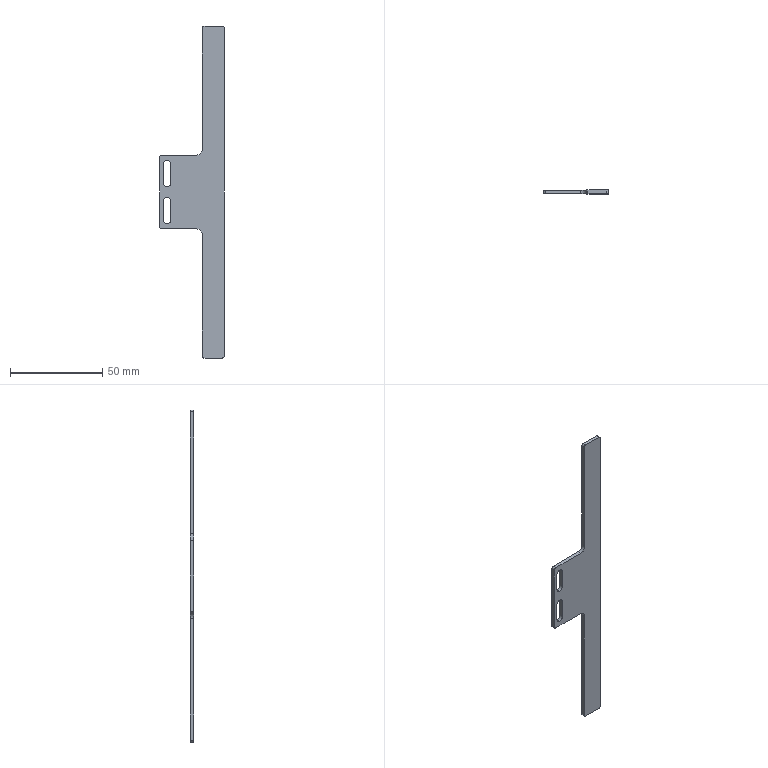Part | NX | features BREP 1 | 1 solid | 28 faces | box 35 x 2 x 180 mm | volume 5942 mm3 | plane 14 | cylinder 14 | commonest cylinder face diameters 2 x6 4.2 x6 6 x2
STEP:
#1=CARTESIAN_POINT('',(-28.9,0.,5.));
#2=VERTEX_POINT('',#1);
#3=CARTESIAN_POINT('',(-28.9,0.,15.));
#4=VERTEX_POINT('',#3);
#5=CARTESIAN_POINT('',(-28.9,0.,15.));
#6=DIRECTION('',(0.,0.,1.));
#7=VECTOR('',#6,1000.);
#8=LINE('',#5,#7);
#9=EDGE_CURVE('',#2,#4,#8,.T.);
#10=ORIENTED_EDGE('',*,*,#9,.T.);
#11=CARTESIAN_POINT('',(-28.9,2.,15.));
#12=VERTEX_POINT('',#11);
#13=CARTESIAN_POINT('',(-28.9,2.,15.));
#14=DIRECTION('',(0.,-1.,0.));
#15=VECTOR('',#14,1000.);
#16=LINE('',#13,#15);
#17=EDGE_CURVE('',#12,#4,#16,.T.);
#18=ORIENTED_EDGE('',*,*,#17,.F.);
#19=CARTESIAN_POINT('',(-28.9,2.,5.));
#20=VERTEX_POINT('',#19);
#21=CARTESIAN_POINT('',(-28.9,2.,15.));
#22=DIRECTION('',(0.,0.,1.));
#23=VECTOR('',#22,1000.);
#24=LINE('',#21,#23);
#25=EDGE_CURVE('',#20,#12,#24,.T.);
#26=ORIENTED_EDGE('',*,*,#25,.F.);
#27=CARTESIAN_POINT('',(-28.9,2.,5.));
#28=DIRECTION('',(0.,-1.,0.));
#29=VECTOR('',#28,1000.);
#30=LINE('',#27,#29);
#31=EDGE_CURVE('',#20,#2,#30,.T.);
#32=ORIENTED_EDGE('',*,*,#31,.T.);
#33=EDGE_LOOP('',(#10,#18,#26,#32));
#34=FACE_BOUND('',#33,.T.);
#35=CARTESIAN_POINT('',(-28.9,2.,15.));
#36=DIRECTION('',(1.,0.,0.));
#37=DIRECTION('',(0.,0.,-1.));
#38=AXIS2_PLACEMENT_3D('',#35,#36,#37);
#39=PLANE('',#38);
#40=ADVANCED_FACE('',(#34),#39,.F.);
#41=CARTESIAN_POINT('',(-33.1,0.,15.));
#42=VERTEX_POINT('',#41);
#43=CARTESIAN_POINT('',(-31.,0.,15.));
#44=DIRECTION('',(0.,-1.,0.));
#45=DIRECTION('',(0.,0.,1.));
#46=AXIS2_PLACEMENT_3D('',#43,#44,#45);
#47=CIRCLE('',#46,2.1);
#48=EDGE_CURVE('',#4,#42,#47,.T.);
#49=ORIENTED_EDGE('',*,*,#48,.T.);
#50=CARTESIAN_POINT('',(-33.1,2.,15.));
#51=VERTEX_POINT('',#50);
#52=CARTESIAN_POINT('',(-33.1,2.,15.));
#53=DIRECTION('',(0.,-1.,0.));
#54=VECTOR('',#53,1000.);
#55=LINE('',#52,#54);
#56=EDGE_CURVE('',#51,#42,#55,.T.);
#57=ORIENTED_EDGE('',*,*,#56,.F.);
#58=CARTESIAN_POINT('',(-31.,2.,15.));
#59=DIRECTION('',(0.,-1.,0.));
#60=DIRECTION('',(0.,0.,1.));
#61=AXIS2_PLACEMENT_3D('',#58,#59,#60);
#62=CIRCLE('',#61,2.1);
#63=EDGE_CURVE('',#12,#51,#62,.T.);
#64=ORIENTED_EDGE('',*,*,#63,.F.);
#65=ORIENTED_EDGE('',*,*,#17,.T.);
#66=EDGE_LOOP('',(#49,#57,#64,#65));
#67=FACE_BOUND('',#66,.T.);
#68=CARTESIAN_POINT('',(-31.,2.,15.));
#69=DIRECTION('',(0.,-1.,0.));
#70=DIRECTION('',(0.,0.,-1.));
#71=AXIS2_PLACEMENT_3D('',#68,#69,#70);
#72=CYLINDRICAL_SURFACE('',#71,2.1);
#73=ADVANCED_FACE('',(#67),#72,.F.);
#74=CARTESIAN_POINT('',(-33.1,0.,5.));
#75=VERTEX_POINT('',#74);
#76=CARTESIAN_POINT('',(-33.1,0.,5.));
#77=DIRECTION('',(0.,0.,-1.));
#78=VECTOR('',#77,1000.);
#79=LINE('',#76,#78);
#80=EDGE_CURVE('',#42,#75,#79,.T.);
#81=ORIENTED_EDGE('',*,*,#80,.T.);
#82=CARTESIAN_POINT('',(-33.1,2.,5.));
#83=VERTEX_POINT('',#82);
#84=CARTESIAN_POINT('',(-33.1,2.,5.));
#85=DIRECTION('',(0.,-1.,0.));
#86=VECTOR('',#85,1000.);
#87=LINE('',#84,#86);
#88=EDGE_CURVE('',#83,#75,#87,.T.);
#89=ORIENTED_EDGE('',*,*,#88,.F.);
#90=CARTESIAN_POINT('',(-33.1,2.,5.));
#91=DIRECTION('',(0.,0.,-1.));
#92=VECTOR('',#91,1000.);
#93=LINE('',#90,#92);
#94=EDGE_CURVE('',#51,#83,#93,.T.);
#95=ORIENTED_EDGE('',*,*,#94,.F.);
#96=ORIENTED_EDGE('',*,*,#56,.T.);
#97=EDGE_LOOP('',(#81,#89,#95,#96));
#98=FACE_BOUND('',#97,.T.);
#99=CARTESIAN_POINT('',(-33.1,2.,5.));
#100=DIRECTION('',(-1.,0.,0.));
#101=DIRECTION('',(0.,0.,1.));
#102=AXIS2_PLACEMENT_3D('',#99,#100,#101);
#103=PLANE('',#102);
#104=ADVANCED_FACE('',(#98),#103,.F.);
#105=CARTESIAN_POINT('',(-31.,2.,2.9));
#106=VERTEX_POINT('',#105);
#107=CARTESIAN_POINT('',(-31.,0.,2.9));
#108=VERTEX_POINT('',#107);
#109=CARTESIAN_POINT('',(-31.,2.,2.9));
#110=DIRECTION('',(0.,-1.,0.));
#111=VECTOR('',#110,1000.);
#112=LINE('',#109,#111);
#113=EDGE_CURVE('',#106,#108,#112,.T.);
#114=ORIENTED_EDGE('',*,*,#113,.F.);
#115=CARTESIAN_POINT('',(-31.,2.,5.));
#116=DIRECTION('',(0.,-1.,0.));
#117=DIRECTION('',(0.,0.,1.));
#118=AXIS2_PLACEMENT_3D('',#115,#116,#117);
#119=CIRCLE('',#118,2.1);
#120=EDGE_CURVE('',#83,#106,#119,.T.);
#121=ORIENTED_EDGE('',*,*,#120,.F.);
#122=ORIENTED_EDGE('',*,*,#88,.T.);
#123=CARTESIAN_POINT('',(-31.,0.,5.));
#124=DIRECTION('',(0.,-1.,0.));
#125=DIRECTION('',(0.,0.,1.));
#126=AXIS2_PLACEMENT_3D('',#123,#124,#125);
#127=CIRCLE('',#126,2.1);
#128=EDGE_CURVE('',#75,#108,#127,.T.);
#129=ORIENTED_EDGE('',*,*,#128,.T.);
#130=EDGE_LOOP('',(#114,#121,#122,#129));
#131=FACE_BOUND('',#130,.T.);
#132=CARTESIAN_POINT('',(-31.,2.,5.));
#133=DIRECTION('',(0.,-1.,0.));
#134=DIRECTION('',(0.,0.,-1.));
#135=AXIS2_PLACEMENT_3D('',#132,#133,#134);
#136=CYLINDRICAL_SURFACE('',#135,2.1);
#137=ADVANCED_FACE('',(#131),#136,.F.);
#138=CARTESIAN_POINT('',(-28.9,0.,-15.));
#139=VERTEX_POINT('',#138);
#140=CARTESIAN_POINT('',(-28.9,0.,-5.));
#141=VERTEX_POINT('',#140);
#142=CARTESIAN_POINT('',(-28.9,0.,-5.));
#143=DIRECTION('',(0.,0.,1.));
#144=VECTOR('',#143,1000.);
#145=LINE('',#142,#144);
#146=EDGE_CURVE('',#139,#141,#145,.T.);
#147=ORIENTED_EDGE('',*,*,#146,.T.);
#148=CARTESIAN_POINT('',(-28.9,2.,-5.));
#149=VERTEX_POINT('',#148);
#150=CARTESIAN_POINT('',(-28.9,2.,-5.));
#151=DIRECTION('',(0.,-1.,0.));
#152=VECTOR('',#151,1000.);
#153=LINE('',#150,#152);
#154=EDGE_CURVE('',#149,#141,#153,.T.);
#155=ORIENTED_EDGE('',*,*,#154,.F.);
#156=CARTESIAN_POINT('',(-28.9,2.,-15.));
#157=VERTEX_POINT('',#156);
#158=CARTESIAN_POINT('',(-28.9,2.,-5.));
#159=DIRECTION('',(0.,0.,1.));
#160=VECTOR('',#159,1000.);
#161=LINE('',#158,#160);
#162=EDGE_CURVE('',#157,#149,#161,.T.);
#163=ORIENTED_EDGE('',*,*,#162,.F.);
#164=CARTESIAN_POINT('',(-28.9,2.,-15.));
#165=DIRECTION('',(0.,-1.,0.));
#166=VECTOR('',#165,1000.);
#167=LINE('',#164,#166);
#168=EDGE_CURVE('',#157,#139,#167,.T.);
#169=ORIENTED_EDGE('',*,*,#168,.T.);
#170=EDGE_LOOP('',(#147,#155,#163,#169));
#171=FACE_BOUND('',#170,.T.);
#172=CARTESIAN_POINT('',(-28.9,2.,-5.));
#173=DIRECTION('',(1.,0.,0.));
#174=DIRECTION('',(0.,0.,-1.));
#175=AXIS2_PLACEMENT_3D('',#172,#173,#174);
#176=PLANE('',#175);
#177=ADVANCED_FACE('',(#171),#176,.F.);
#178=CARTESIAN_POINT('',(-33.1,0.,-5.));
#179=VERTEX_POINT('',#178);
#180=CARTESIAN_POINT('',(-31.,0.,-5.));
#181=DIRECTION('',(0.,-1.,0.));
#182=DIRECTION('',(0.,0.,1.));
#183=AXIS2_PLACEMENT_3D('',#180,#181,#182);
#184=CIRCLE('',#183,2.1);
#185=EDGE_CURVE('',#141,#179,#184,.T.);
#186=ORIENTED_EDGE('',*,*,#185,.T.);
#187=CARTESIAN_POINT('',(-33.1,2.,-5.));
#188=VERTEX_POINT('',#187);
#189=CARTESIAN_POINT('',(-33.1,2.,-5.));
#190=DIRECTION('',(0.,-1.,0.));
#191=VECTOR('',#190,1000.);
#192=LINE('',#189,#191);
#193=EDGE_CURVE('',#188,#179,#192,.T.);
#194=ORIENTED_EDGE('',*,*,#193,.F.);
#195=CARTESIAN_POINT('',(-31.,2.,-5.));
#196=DIRECTION('',(0.,-1.,0.));
#197=DIRECTION('',(0.,0.,1.));
#198=AXIS2_PLACEMENT_3D('',#195,#196,#197);
#199=CIRCLE('',#198,2.1);
#200=EDGE_CURVE('',#149,#188,#199,.T.);
#201=ORIENTED_EDGE('',*,*,#200,.F.);
#202=ORIENTED_EDGE('',*,*,#154,.T.);
#203=EDGE_LOOP('',(#186,#194,#201,#202));
#204=FACE_BOUND('',#203,.T.);
#205=CARTESIAN_POINT('',(-31.,2.,-5.));
#206=DIRECTION('',(0.,-1.,0.));
#207=DIRECTION('',(0.,0.,-1.));
#208=AXIS2_PLACEMENT_3D('',#205,#206,#207);
#209=CYLINDRICAL_SURFACE('',#208,2.1);
#210=ADVANCED_FACE('',(#204),#209,.F.);
#211=CARTESIAN_POINT('',(-33.1,0.,-15.));
#212=VERTEX_POINT('',#211);
#213=CARTESIAN_POINT('',(-33.1,0.,-15.));
#214=DIRECTION('',(0.,0.,-1.));
#215=VECTOR('',#214,1000.);
#216=LINE('',#213,#215);
#217=EDGE_CURVE('',#179,#212,#216,.T.);
#218=ORIENTED_EDGE('',*,*,#217,.T.);
#219=CARTESIAN_POINT('',(-33.1,2.,-15.));
#220=VERTEX_POINT('',#219);
#221=CARTESIAN_POINT('',(-33.1,2.,-15.));
#222=DIRECTION('',(0.,-1.,0.));
#223=VECTOR('',#222,1000.);
#224=LINE('',#221,#223);
#225=EDGE_CURVE('',#220,#212,#224,.T.);
#226=ORIENTED_EDGE('',*,*,#225,.F.);
#227=CARTESIAN_POINT('',(-33.1,2.,-15.));
#228=DIRECTION('',(0.,0.,-1.));
#229=VECTOR('',#228,1000.);
#230=LINE('',#227,#229);
#231=EDGE_CURVE('',#188,#220,#230,.T.);
#232=ORIENTED_EDGE('',*,*,#231,.F.);
#233=ORIENTED_EDGE('',*,*,#193,.T.);
#234=EDGE_LOOP('',(#218,#226,#232,#233));
#235=FACE_BOUND('',#234,.T.);
#236=CARTESIAN_POINT('',(-33.1,2.,-15.));
#237=DIRECTION('',(-1.,0.,0.));
#238=DIRECTION('',(0.,0.,1.));
#239=AXIS2_PLACEMENT_3D('',#236,#237,#238);
#240=PLANE('',#239);
#241=ADVANCED_FACE('',(#235),#240,.F.);
#242=CARTESIAN_POINT('',(-31.,2.,-17.1));
#243=VERTEX_POINT('',#242);
#244=CARTESIAN_POINT('',(-31.,0.,-17.1));
#245=VERTEX_POINT('',#244);
#246=CARTESIAN_POINT('',(-31.,2.,-17.1));
#247=DIRECTION('',(0.,-1.,0.));
#248=VECTOR('',#247,1000.);
#249=LINE('',#246,#248);
#250=EDGE_CURVE('',#243,#245,#249,.T.);
#251=ORIENTED_EDGE('',*,*,#250,.F.);
#252=CARTESIAN_POINT('',(-31.,2.,-15.));
#253=DIRECTION('',(0.,-1.,0.));
#254=DIRECTION('',(0.,0.,1.));
#255=AXIS2_PLACEMENT_3D('',#252,#253,#254);
#256=CIRCLE('',#255,2.1);
#257=EDGE_CURVE('',#220,#243,#256,.T.);
#258=ORIENTED_EDGE('',*,*,#257,.F.);
#259=ORIENTED_EDGE('',*,*,#225,.T.);
#260=CARTESIAN_POINT('',(-31.,0.,-15.));
#261=DIRECTION('',(0.,-1.,0.));
#262=DIRECTION('',(0.,0.,1.));
#263=AXIS2_PLACEMENT_3D('',#260,#261,#262);
#264=CIRCLE('',#263,2.1);
#265=EDGE_CURVE('',#212,#245,#264,.T.);
#266=ORIENTED_EDGE('',*,*,#265,.T.);
#267=EDGE_LOOP('',(#251,#258,#259,#266));
#268=FACE_BOUND('',#267,.T.);
#269=CARTESIAN_POINT('',(-31.,2.,-15.));
#270=DIRECTION('',(0.,-1.,0.));
#271=DIRECTION('',(0.,0.,-1.));
#272=AXIS2_PLACEMENT_3D('',#269,#270,#271);
#273=CYLINDRICAL_SURFACE('',#272,2.1);
#274=ADVANCED_FACE('',(#268),#273,.F.);
#275=CARTESIAN_POINT('',(-35.,0.,-19.));
#276=VERTEX_POINT('',#275);
#277=CARTESIAN_POINT('',(-34.,0.,-20.));
#278=VERTEX_POINT('',#277);
#279=CARTESIAN_POINT('',(-34.,0.,-19.));
#280=DIRECTION('',(0.,-1.,0.));
#281=DIRECTION('',(0.,0.,-1.));
#282=AXIS2_PLACEMENT_3D('',#279,#280,#281);
#283=CIRCLE('',#282,1.);
#284=EDGE_CURVE('',#276,#278,#283,.T.);
#285=ORIENTED_EDGE('',*,*,#284,.T.);
#286=CARTESIAN_POINT('',(-15.,0.,-20.));
#287=VERTEX_POINT('',#286);
#288=CARTESIAN_POINT('',(-34.,0.,-20.));
#289=DIRECTION('',(1.,0.,0.));
#290=VECTOR('',#289,1000.);
#291=LINE('',#288,#290);
#292=EDGE_CURVE('',#278,#287,#291,.T.);
#293=ORIENTED_EDGE('',*,*,#292,.T.);
#294=CARTESIAN_POINT('',(-12.,0.,-23.));
#295=VERTEX_POINT('',#294);
#296=CARTESIAN_POINT('',(-15.,0.,-23.));
#297=DIRECTION('',(0.,1.,0.));
#298=DIRECTION('',(0.,0.,1.));
#299=AXIS2_PLACEMENT_3D('',#296,#297,#298);
#300=CIRCLE('',#299,3.);
#301=EDGE_CURVE('',#287,#295,#300,.T.);
#302=ORIENTED_EDGE('',*,*,#301,.T.);
#303=CARTESIAN_POINT('',(-12.,0.,-89.));
#304=VERTEX_POINT('',#303);
#305=CARTESIAN_POINT('',(-12.,0.,-23.));
#306=DIRECTION('',(0.,0.,-1.));
#307=VECTOR('',#306,1000.);
#308=LINE('',#305,#307);
#309=EDGE_CURVE('',#295,#304,#308,.T.);
#310=ORIENTED_EDGE('',*,*,#309,.T.);
#311=CARTESIAN_POINT('',(-11.,0.,-90.));
#312=VERTEX_POINT('',#311);
#313=CARTESIAN_POINT('',(-11.,0.,-89.));
#314=DIRECTION('',(0.,-1.,0.));
#315=DIRECTION('',(0.,0.,-1.));
#316=AXIS2_PLACEMENT_3D('',#313,#314,#315);
#317=CIRCLE('',#316,1.);
#318=EDGE_CURVE('',#304,#312,#317,.T.);
#319=ORIENTED_EDGE('',*,*,#318,.T.);
#320=CARTESIAN_POINT('',(-1.,0.,-90.));
#321=VERTEX_POINT('',#320);
#322=CARTESIAN_POINT('',(-11.,0.,-90.));
#323=DIRECTION('',(1.,0.,0.));
#324=VECTOR('',#323,1000.);
#325=LINE('',#322,#324);
#326=EDGE_CURVE('',#312,#321,#325,.T.);
#327=ORIENTED_EDGE('',*,*,#326,.T.);
#328=CARTESIAN_POINT('',(0.,0.,-89.));
#329=VERTEX_POINT('',#328);
#330=CARTESIAN_POINT('',(-1.,0.,-89.));
#331=DIRECTION('',(0.,-1.,0.));
#332=DIRECTION('',(0.,0.,-1.));
#333=AXIS2_PLACEMENT_3D('',#330,#331,#332);
#334=CIRCLE('',#333,1.);
#335=EDGE_CURVE('',#321,#329,#334,.T.);
#336=ORIENTED_EDGE('',*,*,#335,.T.);
#337=CARTESIAN_POINT('',(0.,0.,89.));
#338=VERTEX_POINT('',#337);
#339=CARTESIAN_POINT('',(0.,0.,-89.));
#340=DIRECTION('',(0.,0.,1.));
#341=VECTOR('',#340,1000.);
#342=LINE('',#339,#341);
#343=EDGE_CURVE('',#329,#338,#342,.T.);
#344=ORIENTED_EDGE('',*,*,#343,.T.);
#345=CARTESIAN_POINT('',(-1.,0.,90.));
#346=VERTEX_POINT('',#345);
#347=CARTESIAN_POINT('',(-1.,0.,89.));
#348=DIRECTION('',(0.,-1.,0.));
#349=DIRECTION('',(0.,0.,-1.));
#350=AXIS2_PLACEMENT_3D('',#347,#348,#349);
#351=CIRCLE('',#350,1.);
#352=EDGE_CURVE('',#338,#346,#351,.T.);
#353=ORIENTED_EDGE('',*,*,#352,.T.);
#354=CARTESIAN_POINT('',(-11.,0.,90.));
#355=VERTEX_POINT('',#354);
#356=CARTESIAN_POINT('',(-1.,0.,90.));
#357=DIRECTION('',(-1.,0.,0.));
#358=VECTOR('',#357,1000.);
#359=LINE('',#356,#358);
#360=EDGE_CURVE('',#346,#355,#359,.T.);
#361=ORIENTED_EDGE('',*,*,#360,.T.);
#362=CARTESIAN_POINT('',(-12.,0.,89.));
#363=VERTEX_POINT('',#362);
#364=CARTESIAN_POINT('',(-11.,0.,89.));
#365=DIRECTION('',(0.,-1.,0.));
#366=DIRECTION('',(0.,0.,-1.));
#367=AXIS2_PLACEMENT_3D('',#364,#365,#366);
#368=CIRCLE('',#367,1.);
#369=EDGE_CURVE('',#355,#363,#368,.T.);
#370=ORIENTED_EDGE('',*,*,#369,.T.);
#371=CARTESIAN_POINT('',(-12.,0.,23.));
#372=VERTEX_POINT('',#371);
#373=CARTESIAN_POINT('',(-12.,0.,89.));
#374=DIRECTION('',(0.,0.,-1.));
#375=VECTOR('',#374,1000.);
#376=LINE('',#373,#375);
#377=EDGE_CURVE('',#363,#372,#376,.T.);
#378=ORIENTED_EDGE('',*,*,#377,.T.);
#379=CARTESIAN_POINT('',(-15.,0.,20.));
#380=VERTEX_POINT('',#379);
#381=CARTESIAN_POINT('',(-15.,0.,23.));
#382=DIRECTION('',(0.,1.,0.));
#383=DIRECTION('',(0.,0.,1.));
#384=AXIS2_PLACEMENT_3D('',#381,#382,#383);
#385=CIRCLE('',#384,3.);
#386=EDGE_CURVE('',#372,#380,#385,.T.);
#387=ORIENTED_EDGE('',*,*,#386,.T.);
#388=CARTESIAN_POINT('',(-34.,0.,20.));
#389=VERTEX_POINT('',#388);
#390=CARTESIAN_POINT('',(-15.,0.,20.));
#391=DIRECTION('',(-1.,0.,0.));
#392=VECTOR('',#391,1000.);
#393=LINE('',#390,#392);
#394=EDGE_CURVE('',#380,#389,#393,.T.);
#395=ORIENTED_EDGE('',*,*,#394,.T.);
#396=CARTESIAN_POINT('',(-35.,0.,19.));
#397=VERTEX_POINT('',#396);
#398=CARTESIAN_POINT('',(-34.,0.,19.));
#399=DIRECTION('',(0.,-1.,0.));
#400=DIRECTION('',(0.,0.,-1.));
#401=AXIS2_PLACEMENT_3D('',#398,#399,#400);
#402=CIRCLE('',#401,1.);
#403=EDGE_CURVE('',#389,#397,#402,.T.);
#404=ORIENTED_EDGE('',*,*,#403,.T.);
#405=CARTESIAN_POINT('',(-35.,0.,19.));
#406=DIRECTION('',(0.,0.,-1.));
#407=VECTOR('',#406,1000.);
#408=LINE('',#405,#407);
#409=EDGE_CURVE('',#397,#276,#408,.T.);
#410=ORIENTED_EDGE('',*,*,#409,.T.);
#411=EDGE_LOOP('',(#285,#293,#302,#310,#319,#327,#336,#344,#353,#361,#370,#378,#387,#395,#404,#410));
#412=FACE_BOUND('',#411,.T.);
#413=ORIENTED_EDGE('',*,*,#265,.F.);
#414=ORIENTED_EDGE('',*,*,#217,.F.);
#415=ORIENTED_EDGE('',*,*,#185,.F.);
#416=ORIENTED_EDGE('',*,*,#146,.F.);
#417=CARTESIAN_POINT('',(-31.,0.,-15.));
#418=DIRECTION('',(0.,-1.,0.));
#419=DIRECTION('',(0.,0.,1.));
#420=AXIS2_PLACEMENT_3D('',#417,#418,#419);
#421=CIRCLE('',#420,2.1);
#422=EDGE_CURVE('',#245,#139,#421,.T.);
#423=ORIENTED_EDGE('',*,*,#422,.F.);
#424=EDGE_LOOP('',(#413,#414,#415,#416,#423));
#425=FACE_BOUND('',#424,.T.);
#426=ORIENTED_EDGE('',*,*,#128,.F.);
#427=ORIENTED_EDGE('',*,*,#80,.F.);
#428=ORIENTED_EDGE('',*,*,#48,.F.);
#429=ORIENTED_EDGE('',*,*,#9,.F.);
#430=CARTESIAN_POINT('',(-31.,0.,5.));
#431=DIRECTION('',(0.,-1.,0.));
#432=DIRECTION('',(0.,0.,1.));
#433=AXIS2_PLACEMENT_3D('',#430,#431,#432);
#434=CIRCLE('',#433,2.1);
#435=EDGE_CURVE('',#108,#2,#434,.T.);
#436=ORIENTED_EDGE('',*,*,#435,.F.);
#437=EDGE_LOOP('',(#426,#427,#428,#429,#436));
#438=FACE_BOUND('',#437,.T.);
#439=CARTESIAN_POINT('',(-34.,0.,-19.));
#440=DIRECTION('',(0.,-1.,0.));
#441=DIRECTION('',(0.,0.,-1.));
#442=AXIS2_PLACEMENT_3D('',#439,#440,#441);
#443=PLANE('',#442);
#444=ADVANCED_FACE('',(#412,#425,#438),#443,.T.);
#445=CARTESIAN_POINT('',(-35.,2.,-19.));
#446=VERTEX_POINT('',#445);
#447=CARTESIAN_POINT('',(-34.,2.,-20.));
#448=VERTEX_POINT('',#447);
#449=CARTESIAN_POINT('',(-34.,2.,-19.));
#450=DIRECTION('',(0.,-1.,0.));
#451=DIRECTION('',(0.,0.,-1.));
#452=AXIS2_PLACEMENT_3D('',#449,#450,#451);
#453=CIRCLE('',#452,1.);
#454=EDGE_CURVE('',#446,#448,#453,.T.);
#455=ORIENTED_EDGE('',*,*,#454,.F.);
#456=CARTESIAN_POINT('',(-35.,2.,19.));
#457=VERTEX_POINT('',#456);
#458=CARTESIAN_POINT('',(-35.,2.,19.));
#459=DIRECTION('',(0.,0.,-1.));
#460=VECTOR('',#459,1000.);
#461=LINE('',#458,#460);
#462=EDGE_CURVE('',#457,#446,#461,.T.);
#463=ORIENTED_EDGE('',*,*,#462,.F.);
#464=CARTESIAN_POINT('',(-34.,2.,20.));
#465=VERTEX_POINT('',#464);
#466=CARTESIAN_POINT('',(-34.,2.,19.));
#467=DIRECTION('',(0.,-1.,0.));
#468=DIRECTION('',(0.,0.,-1.));
#469=AXIS2_PLACEMENT_3D('',#466,#467,#468);
#470=CIRCLE('',#469,1.);
#471=EDGE_CURVE('',#465,#457,#470,.T.);
#472=ORIENTED_EDGE('',*,*,#471,.F.);
#473=CARTESIAN_POINT('',(-15.,2.,20.));
#474=VERTEX_POINT('',#473);
#475=CARTESIAN_POINT('',(-15.,2.,20.));
#476=DIRECTION('',(-1.,0.,0.));
#477=VECTOR('',#476,1000.);
#478=LINE('',#475,#477);
#479=EDGE_CURVE('',#474,#465,#478,.T.);
#480=ORIENTED_EDGE('',*,*,#479,.F.);
#481=CARTESIAN_POINT('',(-12.,2.,23.));
#482=VERTEX_POINT('',#481);
#483=CARTESIAN_POINT('',(-15.,2.,23.));
#484=DIRECTION('',(0.,1.,0.));
#485=DIRECTION('',(0.,0.,1.));
#486=AXIS2_PLACEMENT_3D('',#483,#484,#485);
#487=CIRCLE('',#486,3.);
#488=EDGE_CURVE('',#482,#474,#487,.T.);
#489=ORIENTED_EDGE('',*,*,#488,.F.);
#490=CARTESIAN_POINT('',(-12.,2.,89.));
#491=VERTEX_POINT('',#490);
#492=CARTESIAN_POINT('',(-12.,2.,89.));
#493=DIRECTION('',(0.,0.,-1.));
#494=VECTOR('',#493,1000.);
#495=LINE('',#492,#494);
#496=EDGE_CURVE('',#491,#482,#495,.T.);
#497=ORIENTED_EDGE('',*,*,#496,.F.);
#498=CARTESIAN_POINT('',(-11.,2.,90.));
#499=VERTEX_POINT('',#498);
#500=CARTESIAN_POINT('',(-11.,2.,89.));
#501=DIRECTION('',(0.,-1.,0.));
#502=DIRECTION('',(0.,0.,-1.));
#503=AXIS2_PLACEMENT_3D('',#500,#501,#502);
#504=CIRCLE('',#503,1.);
#505=EDGE_CURVE('',#499,#491,#504,.T.);
#506=ORIENTED_EDGE('',*,*,#505,.F.);
#507=CARTESIAN_POINT('',(-1.,2.,90.));
#508=VERTEX_POINT('',#507);
#509=CARTESIAN_POINT('',(-1.,2.,90.));
#510=DIRECTION('',(-1.,0.,0.));
#511=VECTOR('',#510,1000.);
#512=LINE('',#509,#511);
#513=EDGE_CURVE('',#508,#499,#512,.T.);
#514=ORIENTED_EDGE('',*,*,#513,.F.);
#515=CARTESIAN_POINT('',(0.,2.,89.));
#516=VERTEX_POINT('',#515);
#517=CARTESIAN_POINT('',(-1.,2.,89.));
#518=DIRECTION('',(0.,-1.,0.));
#519=DIRECTION('',(0.,0.,-1.));
#520=AXIS2_PLACEMENT_3D('',#517,#518,#519);
#521=CIRCLE('',#520,1.);
#522=EDGE_CURVE('',#516,#508,#521,.T.);
#523=ORIENTED_EDGE('',*,*,#522,.F.);
#524=CARTESIAN_POINT('',(0.,2.,-89.));
#525=VERTEX_POINT('',#524);
#526=CARTESIAN_POINT('',(0.,2.,-89.));
#527=DIRECTION('',(0.,0.,1.));
#528=VECTOR('',#527,1000.);
#529=LINE('',#526,#528);
#530=EDGE_CURVE('',#525,#516,#529,.T.);
#531=ORIENTED_EDGE('',*,*,#530,.F.);
#532=CARTESIAN_POINT('',(-1.,2.,-90.));
#533=VERTEX_POINT('',#532);
#534=CARTESIAN_POINT('',(-1.,2.,-89.));
#535=DIRECTION('',(0.,-1.,0.));
#536=DIRECTION('',(0.,0.,-1.));
#537=AXIS2_PLACEMENT_3D('',#534,#535,#536);
#538=CIRCLE('',#537,1.);
#539=EDGE_CURVE('',#533,#525,#538,.T.);
#540=ORIENTED_EDGE('',*,*,#539,.F.);
#541=CARTESIAN_POINT('',(-11.,2.,-90.));
#542=VERTEX_POINT('',#541);
#543=CARTESIAN_POINT('',(-11.,2.,-90.));
#544=DIRECTION('',(1.,0.,0.));
#545=VECTOR('',#544,1000.);
#546=LINE('',#543,#545);
#547=EDGE_CURVE('',#542,#533,#546,.T.);
#548=ORIENTED_EDGE('',*,*,#547,.F.);
#549=CARTESIAN_POINT('',(-12.,2.,-89.));
#550=VERTEX_POINT('',#549);
#551=CARTESIAN_POINT('',(-11.,2.,-89.));
#552=DIRECTION('',(0.,-1.,0.));
#553=DIRECTION('',(0.,0.,-1.));
#554=AXIS2_PLACEMENT_3D('',#551,#552,#553);
#555=CIRCLE('',#554,1.);
#556=EDGE_CURVE('',#550,#542,#555,.T.);
#557=ORIENTED_EDGE('',*,*,#556,.F.);
#558=CARTESIAN_POINT('',(-12.,2.,-23.));
#559=VERTEX_POINT('',#558);
#560=CARTESIAN_POINT('',(-12.,2.,-23.));
#561=DIRECTION('',(0.,0.,-1.));
#562=VECTOR('',#561,1000.);
#563=LINE('',#560,#562);
#564=EDGE_CURVE('',#559,#550,#563,.T.);
#565=ORIENTED_EDGE('',*,*,#564,.F.);
#566=CARTESIAN_POINT('',(-15.,2.,-20.));
#567=VERTEX_POINT('',#566);
#568=CARTESIAN_POINT('',(-15.,2.,-23.));
#569=DIRECTION('',(0.,1.,0.));
#570=DIRECTION('',(0.,0.,1.));
#571=AXIS2_PLACEMENT_3D('',#568,#569,#570);
#572=CIRCLE('',#571,3.);
#573=EDGE_CURVE('',#567,#559,#572,.T.);
#574=ORIENTED_EDGE('',*,*,#573,.F.);
#575=CARTESIAN_POINT('',(-34.,2.,-20.));
#576=DIRECTION('',(1.,0.,0.));
#577=VECTOR('',#576,1000.);
#578=LINE('',#575,#577);
#579=EDGE_CURVE('',#448,#567,#578,.T.);
#580=ORIENTED_EDGE('',*,*,#579,.F.);
#581=EDGE_LOOP('',(#455,#463,#472,#480,#489,#497,#506,#514,#523,#531,#540,#548,#557,#565,#574,#580));
#582=FACE_BOUND('',#581,.T.);
#583=ORIENTED_EDGE('',*,*,#231,.T.);
#584=ORIENTED_EDGE('',*,*,#257,.T.);
#585=CARTESIAN_POINT('',(-31.,2.,-15.));
#586=DIRECTION('',(0.,-1.,0.));
#587=DIRECTION('',(0.,0.,1.));
#588=AXIS2_PLACEMENT_3D('',#585,#586,#587);
#589=CIRCLE('',#588,2.1);
#590=EDGE_CURVE('',#243,#157,#589,.T.);
#591=ORIENTED_EDGE('',*,*,#590,.T.);
#592=ORIENTED_EDGE('',*,*,#162,.T.);
#593=ORIENTED_EDGE('',*,*,#200,.T.);
#594=EDGE_LOOP('',(#583,#584,#591,#592,#593));
#595=FACE_BOUND('',#594,.T.);
#596=ORIENTED_EDGE('',*,*,#94,.T.);
#597=ORIENTED_EDGE('',*,*,#120,.T.);
#598=CARTESIAN_POINT('',(-31.,2.,5.));
#599=DIRECTION('',(0.,-1.,0.));
#600=DIRECTION('',(0.,0.,1.));
#601=AXIS2_PLACEMENT_3D('',#598,#599,#600);
#602=CIRCLE('',#601,2.1);
#603=EDGE_CURVE('',#106,#20,#602,.T.);
#604=ORIENTED_EDGE('',*,*,#603,.T.);
#605=ORIENTED_EDGE('',*,*,#25,.T.);
#606=ORIENTED_EDGE('',*,*,#63,.T.);
#607=EDGE_LOOP('',(#596,#597,#604,#605,#606));
#608=FACE_BOUND('',#607,.T.);
#609=CARTESIAN_POINT('',(-34.,2.,-19.));
#610=DIRECTION('',(0.,-1.,0.));
#611=DIRECTION('',(0.,0.,-1.));
#612=AXIS2_PLACEMENT_3D('',#609,#610,#611);
#613=PLANE('',#612);
#614=ADVANCED_FACE('',(#582,#595,#608),#613,.F.);
#615=ORIENTED_EDGE('',*,*,#292,.F.);
#616=CARTESIAN_POINT('',(-34.,2.,-20.));
#617=DIRECTION('',(0.,-1.,0.));
#618=VECTOR('',#617,1000.);
#619=LINE('',#616,#618);
#620=EDGE_CURVE('',#448,#278,#619,.T.);
#621=ORIENTED_EDGE('',*,*,#620,.F.);
#622=ORIENTED_EDGE('',*,*,#579,.T.);
#623=CARTESIAN_POINT('',(-15.,2.,-20.));
#624=DIRECTION('',(0.,-1.,0.));
#625=VECTOR('',#624,1000.);
#626=LINE('',#623,#625);
#627=EDGE_CURVE('',#567,#287,#626,.T.);
#628=ORIENTED_EDGE('',*,*,#627,.T.);
#629=EDGE_LOOP('',(#615,#621,#622,#628));
#630=FACE_BOUND('',#629,.T.);
#631=CARTESIAN_POINT('',(-34.,2.,-20.));
#632=DIRECTION('',(0.,0.,-1.));
#633=DIRECTION('',(-1.,0.,0.));
#634=AXIS2_PLACEMENT_3D('',#631,#632,#633);
#635=PLANE('',#634);
#636=ADVANCED_FACE('',(#630),#635,.T.);
#637=ORIENTED_EDGE('',*,*,#301,.F.);
#638=ORIENTED_EDGE('',*,*,#627,.F.);
#639=ORIENTED_EDGE('',*,*,#573,.T.);
#640=CARTESIAN_POINT('',(-12.,2.,-23.));
#641=DIRECTION('',(0.,-1.,0.));
#642=VECTOR('',#641,1000.);
#643=LINE('',#640,#642);
#644=EDGE_CURVE('',#559,#295,#643,.T.);
#645=ORIENTED_EDGE('',*,*,#644,.T.);
#646=EDGE_LOOP('',(#637,#638,#639,#645));
#647=FACE_BOUND('',#646,.T.);
#648=CARTESIAN_POINT('',(-15.,2.,-23.));
#649=DIRECTION('',(0.,-1.,0.));
#650=DIRECTION('',(0.,0.,-1.));
#651=AXIS2_PLACEMENT_3D('',#648,#649,#650);
#652=CYLINDRICAL_SURFACE('',#651,3.);
#653=ADVANCED_FACE('',(#647),#652,.F.);
#654=ORIENTED_EDGE('',*,*,#309,.F.);
#655=ORIENTED_EDGE('',*,*,#644,.F.);
#656=ORIENTED_EDGE('',*,*,#564,.T.);
#657=CARTESIAN_POINT('',(-12.,2.,-89.));
#658=DIRECTION('',(0.,-1.,0.));
#659=VECTOR('',#658,1000.);
#660=LINE('',#657,#659);
#661=EDGE_CURVE('',#550,#304,#660,.T.);
#662=ORIENTED_EDGE('',*,*,#661,.T.);
#663=EDGE_LOOP('',(#654,#655,#656,#662));
#664=FACE_BOUND('',#663,.T.);
#665=CARTESIAN_POINT('',(-12.,2.,-23.));
#666=DIRECTION('',(-1.,0.,0.));
#667=DIRECTION('',(0.,0.,1.));
#668=AXIS2_PLACEMENT_3D('',#665,#666,#667);
#669=PLANE('',#668);
#670=ADVANCED_FACE('',(#664),#669,.T.);
#671=ORIENTED_EDGE('',*,*,#318,.F.);
#672=ORIENTED_EDGE('',*,*,#661,.F.);
#673=ORIENTED_EDGE('',*,*,#556,.T.);
#674=CARTESIAN_POINT('',(-11.,2.,-90.));
#675=DIRECTION('',(0.,-1.,0.));
#676=VECTOR('',#675,1000.);
#677=LINE('',#674,#676);
#678=EDGE_CURVE('',#542,#312,#677,.T.);
#679=ORIENTED_EDGE('',*,*,#678,.T.);
#680=EDGE_LOOP('',(#671,#672,#673,#679));
#681=FACE_BOUND('',#680,.T.);
#682=CARTESIAN_POINT('',(-11.,2.,-89.));
#683=DIRECTION('',(0.,-1.,0.));
#684=DIRECTION('',(0.,0.,-1.));
#685=AXIS2_PLACEMENT_3D('',#682,#683,#684);
#686=CYLINDRICAL_SURFACE('',#685,1.);
#687=ADVANCED_FACE('',(#681),#686,.T.);
#688=ORIENTED_EDGE('',*,*,#326,.F.);
#689=ORIENTED_EDGE('',*,*,#678,.F.);
#690=ORIENTED_EDGE('',*,*,#547,.T.);
#691=CARTESIAN_POINT('',(-1.,2.,-90.));
#692=DIRECTION('',(0.,-1.,0.));
#693=VECTOR('',#692,1000.);
#694=LINE('',#691,#693);
#695=EDGE_CURVE('',#533,#321,#694,.T.);
#696=ORIENTED_EDGE('',*,*,#695,.T.);
#697=EDGE_LOOP('',(#688,#689,#690,#696));
#698=FACE_BOUND('',#697,.T.);
#699=CARTESIAN_POINT('',(-11.,2.,-90.));
#700=DIRECTION('',(0.,0.,-1.));
#701=DIRECTION('',(-1.,0.,0.));
#702=AXIS2_PLACEMENT_3D('',#699,#700,#701);
#703=PLANE('',#702);
#704=ADVANCED_FACE('',(#698),#703,.T.);
#705=ORIENTED_EDGE('',*,*,#335,.F.);
#706=ORIENTED_EDGE('',*,*,#695,.F.);
#707=ORIENTED_EDGE('',*,*,#539,.T.);
#708=CARTESIAN_POINT('',(0.,2.,-89.));
#709=DIRECTION('',(0.,-1.,0.));
#710=VECTOR('',#709,1000.);
#711=LINE('',#708,#710);
#712=EDGE_CURVE('',#525,#329,#711,.T.);
#713=ORIENTED_EDGE('',*,*,#712,.T.);
#714=EDGE_LOOP('',(#705,#706,#707,#713));
#715=FACE_BOUND('',#714,.T.);
#716=CARTESIAN_POINT('',(-1.,2.,-89.));
#717=DIRECTION('',(0.,-1.,0.));
#718=DIRECTION('',(0.,0.,-1.));
#719=AXIS2_PLACEMENT_3D('',#716,#717,#718);
#720=CYLINDRICAL_SURFACE('',#719,1.);
#721=ADVANCED_FACE('',(#715),#720,.T.);
#722=ORIENTED_EDGE('',*,*,#343,.F.);
#723=ORIENTED_EDGE('',*,*,#712,.F.);
#724=ORIENTED_EDGE('',*,*,#530,.T.);
#725=CARTESIAN_POINT('',(0.,2.,89.));
#726=DIRECTION('',(0.,-1.,0.));
#727=VECTOR('',#726,1000.);
#728=LINE('',#725,#727);
#729=EDGE_CURVE('',#516,#338,#728,.T.);
#730=ORIENTED_EDGE('',*,*,#729,.T.);
#731=EDGE_LOOP('',(#722,#723,#724,#730));
#732=FACE_BOUND('',#731,.T.);
#733=CARTESIAN_POINT('',(0.,2.,-89.));
#734=DIRECTION('',(1.,0.,0.));
#735=DIRECTION('',(0.,0.,-1.));
#736=AXIS2_PLACEMENT_3D('',#733,#734,#735);
#737=PLANE('',#736);
#738=ADVANCED_FACE('',(#732),#737,.T.);
#739=ORIENTED_EDGE('',*,*,#352,.F.);
#740=ORIENTED_EDGE('',*,*,#729,.F.);
#741=ORIENTED_EDGE('',*,*,#522,.T.);
#742=CARTESIAN_POINT('',(-1.,2.,90.));
#743=DIRECTION('',(0.,-1.,0.));
#744=VECTOR('',#743,1000.);
#745=LINE('',#742,#744);
#746=EDGE_CURVE('',#508,#346,#745,.T.);
#747=ORIENTED_EDGE('',*,*,#746,.T.);
#748=EDGE_LOOP('',(#739,#740,#741,#747));
#749=FACE_BOUND('',#748,.T.);
#750=CARTESIAN_POINT('',(-1.,2.,89.));
#751=DIRECTION('',(0.,-1.,0.));
#752=DIRECTION('',(0.,0.,-1.));
#753=AXIS2_PLACEMENT_3D('',#750,#751,#752);
#754=CYLINDRICAL_SURFACE('',#753,1.);
#755=ADVANCED_FACE('',(#749),#754,.T.);
#756=ORIENTED_EDGE('',*,*,#360,.F.);
#757=ORIENTED_EDGE('',*,*,#746,.F.);
#758=ORIENTED_EDGE('',*,*,#513,.T.);
#759=CARTESIAN_POINT('',(-11.,2.,90.));
#760=DIRECTION('',(0.,-1.,0.));
#761=VECTOR('',#760,1000.);
#762=LINE('',#759,#761);
#763=EDGE_CURVE('',#499,#355,#762,.T.);
#764=ORIENTED_EDGE('',*,*,#763,.T.);
#765=EDGE_LOOP('',(#756,#757,#758,#764));
#766=FACE_BOUND('',#765,.T.);
#767=CARTESIAN_POINT('',(-1.,2.,90.));
#768=DIRECTION('',(0.,0.,1.));
#769=DIRECTION('',(1.,0.,0.));
#770=AXIS2_PLACEMENT_3D('',#767,#768,#769);
#771=PLANE('',#770);
#772=ADVANCED_FACE('',(#766),#771,.T.);
#773=ORIENTED_EDGE('',*,*,#369,.F.);
#774=ORIENTED_EDGE('',*,*,#763,.F.);
#775=ORIENTED_EDGE('',*,*,#505,.T.);
#776=CARTESIAN_POINT('',(-12.,2.,89.));
#777=DIRECTION('',(0.,-1.,0.));
#778=VECTOR('',#777,1000.);
#779=LINE('',#776,#778);
#780=EDGE_CURVE('',#491,#363,#779,.T.);
#781=ORIENTED_EDGE('',*,*,#780,.T.);
#782=EDGE_LOOP('',(#773,#774,#775,#781));
#783=FACE_BOUND('',#782,.T.);
#784=CARTESIAN_POINT('',(-11.,2.,89.));
#785=DIRECTION('',(0.,-1.,0.));
#786=DIRECTION('',(0.,0.,-1.));
#787=AXIS2_PLACEMENT_3D('',#784,#785,#786);
#788=CYLINDRICAL_SURFACE('',#787,1.);
#789=ADVANCED_FACE('',(#783),#788,.T.);
#790=ORIENTED_EDGE('',*,*,#377,.F.);
#791=ORIENTED_EDGE('',*,*,#780,.F.);
#792=ORIENTED_EDGE('',*,*,#496,.T.);
#793=CARTESIAN_POINT('',(-12.,2.,23.));
#794=DIRECTION('',(0.,-1.,0.));
#795=VECTOR('',#794,1000.);
#796=LINE('',#793,#795);
#797=EDGE_CURVE('',#482,#372,#796,.T.);
#798=ORIENTED_EDGE('',*,*,#797,.T.);
#799=EDGE_LOOP('',(#790,#791,#792,#798));
#800=FACE_BOUND('',#799,.T.);
#801=CARTESIAN_POINT('',(-12.,2.,89.));
#802=DIRECTION('',(-1.,0.,0.));
#803=DIRECTION('',(0.,0.,1.));
#804=AXIS2_PLACEMENT_3D('',#801,#802,#803);
#805=PLANE('',#804);
#806=ADVANCED_FACE('',(#800),#805,.T.);
#807=ORIENTED_EDGE('',*,*,#386,.F.);
#808=ORIENTED_EDGE('',*,*,#797,.F.);
#809=ORIENTED_EDGE('',*,*,#488,.T.);
#810=CARTESIAN_POINT('',(-15.,2.,20.));
#811=DIRECTION('',(0.,-1.,0.));
#812=VECTOR('',#811,1000.);
#813=LINE('',#810,#812);
#814=EDGE_CURVE('',#474,#380,#813,.T.);
#815=ORIENTED_EDGE('',*,*,#814,.T.);
#816=EDGE_LOOP('',(#807,#808,#809,#815));
#817=FACE_BOUND('',#816,.T.);
#818=CARTESIAN_POINT('',(-15.,2.,23.));
#819=DIRECTION('',(0.,-1.,0.));
#820=DIRECTION('',(0.,0.,-1.));
#821=AXIS2_PLACEMENT_3D('',#818,#819,#820);
#822=CYLINDRICAL_SURFACE('',#821,3.);
#823=ADVANCED_FACE('',(#817),#822,.F.);
#824=ORIENTED_EDGE('',*,*,#394,.F.);
#825=ORIENTED_EDGE('',*,*,#814,.F.);
#826=ORIENTED_EDGE('',*,*,#479,.T.);
#827=CARTESIAN_POINT('',(-34.,2.,20.));
#828=DIRECTION('',(0.,-1.,0.));
#829=VECTOR('',#828,1000.);
#830=LINE('',#827,#829);
#831=EDGE_CURVE('',#465,#389,#830,.T.);
#832=ORIENTED_EDGE('',*,*,#831,.T.);
#833=EDGE_LOOP('',(#824,#825,#826,#832));
#834=FACE_BOUND('',#833,.T.);
#835=CARTESIAN_POINT('',(-15.,2.,20.));
#836=DIRECTION('',(0.,0.,1.));
#837=DIRECTION('',(1.,0.,0.));
#838=AXIS2_PLACEMENT_3D('',#835,#836,#837);
#839=PLANE('',#838);
#840=ADVANCED_FACE('',(#834),#839,.T.);
#841=ORIENTED_EDGE('',*,*,#403,.F.);
#842=ORIENTED_EDGE('',*,*,#831,.F.);
#843=ORIENTED_EDGE('',*,*,#471,.T.);
#844=CARTESIAN_POINT('',(-35.,2.,19.));
#845=DIRECTION('',(0.,-1.,0.));
#846=VECTOR('',#845,1000.);
#847=LINE('',#844,#846);
#848=EDGE_CURVE('',#457,#397,#847,.T.);
#849=ORIENTED_EDGE('',*,*,#848,.T.);
#850=EDGE_LOOP('',(#841,#842,#843,#849));
#851=FACE_BOUND('',#850,.T.);
#852=CARTESIAN_POINT('',(-34.,2.,19.));
#853=DIRECTION('',(0.,-1.,0.));
#854=DIRECTION('',(0.,0.,-1.));
#855=AXIS2_PLACEMENT_3D('',#852,#853,#854);
#856=CYLINDRICAL_SURFACE('',#855,1.);
#857=ADVANCED_FACE('',(#851),#856,.T.);
#858=ORIENTED_EDGE('',*,*,#409,.F.);
#859=ORIENTED_EDGE('',*,*,#848,.F.);
#860=ORIENTED_EDGE('',*,*,#462,.T.);
#861=CARTESIAN_POINT('',(-35.,2.,-19.));
#862=DIRECTION('',(0.,-1.,0.));
#863=VECTOR('',#862,1000.);
#864=LINE('',#861,#863);
#865=EDGE_CURVE('',#446,#276,#864,.T.);
#866=ORIENTED_EDGE('',*,*,#865,.T.);
#867=EDGE_LOOP('',(#858,#859,#860,#866));
#868=FACE_BOUND('',#867,.T.);
#869=CARTESIAN_POINT('',(-35.,2.,19.));
#870=DIRECTION('',(-1.,0.,0.));
#871=DIRECTION('',(0.,0.,1.));
#872=AXIS2_PLACEMENT_3D('',#869,#870,#871);
#873=PLANE('',#872);
#874=ADVANCED_FACE('',(#868),#873,.T.);
#875=ORIENTED_EDGE('',*,*,#284,.F.);
#876=ORIENTED_EDGE('',*,*,#865,.F.);
#877=ORIENTED_EDGE('',*,*,#454,.T.);
#878=ORIENTED_EDGE('',*,*,#620,.T.);
#879=EDGE_LOOP('',(#875,#876,#877,#878));
#880=FACE_BOUND('',#879,.T.);
#881=CARTESIAN_POINT('',(-34.,2.,-19.));
#882=DIRECTION('',(0.,-1.,0.));
#883=DIRECTION('',(0.,0.,-1.));
#884=AXIS2_PLACEMENT_3D('',#881,#882,#883);
#885=CYLINDRICAL_SURFACE('',#884,1.);
#886=ADVANCED_FACE('',(#880),#885,.T.);
#887=ORIENTED_EDGE('',*,*,#590,.F.);
#888=ORIENTED_EDGE('',*,*,#250,.T.);
#889=ORIENTED_EDGE('',*,*,#422,.T.);
#890=ORIENTED_EDGE('',*,*,#168,.F.);
#891=EDGE_LOOP('',(#887,#888,#889,#890));
#892=FACE_BOUND('',#891,.T.);
#893=CARTESIAN_POINT('',(-31.,2.,-15.));
#894=DIRECTION('',(0.,-1.,0.));
#895=DIRECTION('',(0.,0.,-1.));
#896=AXIS2_PLACEMENT_3D('',#893,#894,#895);
#897=CYLINDRICAL_SURFACE('',#896,2.1);
#898=ADVANCED_FACE('',(#892),#897,.F.);
#899=ORIENTED_EDGE('',*,*,#603,.F.);
#900=ORIENTED_EDGE('',*,*,#113,.T.);
#901=ORIENTED_EDGE('',*,*,#435,.T.);
#902=ORIENTED_EDGE('',*,*,#31,.F.);
#903=EDGE_LOOP('',(#899,#900,#901,#902));
#904=FACE_BOUND('',#903,.T.);
#905=CARTESIAN_POINT('',(-31.,2.,5.));
#906=DIRECTION('',(0.,-1.,0.));
#907=DIRECTION('',(0.,0.,-1.));
#908=AXIS2_PLACEMENT_3D('',#905,#906,#907);
#909=CYLINDRICAL_SURFACE('',#908,2.1);
#910=ADVANCED_FACE('',(#904),#909,.F.);
#911=CLOSED_SHELL('',(#40,#73,#104,#137,#177,#210,#241,#274,#444,#614,#636,#653,#670,#687,#704,#721,#738,#755,#772,#789,#806,#823,#840,#857,#874,#886,#898,#910));
#912=MANIFOLD_SOLID_BREP('',#911);
#913=(LENGTH_UNIT()NAMED_UNIT(*)SI_UNIT(.MILLI.,.METRE.));
#914=UNCERTAINTY_MEASURE_WITH_UNIT(LENGTH_MEASURE(0.00001),#913,'','');
#915=(NAMED_UNIT(*)PLANE_ANGLE_UNIT()SI_UNIT($,.RADIAN.));
#916=(NAMED_UNIT(*)SI_UNIT($,.STERADIAN.)SOLID_ANGLE_UNIT());
#917=(GEOMETRIC_REPRESENTATION_CONTEXT(3)GLOBAL_UNCERTAINTY_ASSIGNED_CONTEXT((#914))GLOBAL_UNIT_ASSIGNED_CONTEXT((#913,#915,#916))REPRESENTATION_CONTEXT('',''));
#918=ADVANCED_BREP_SHAPE_REPRESENTATION('',(#912),#917);